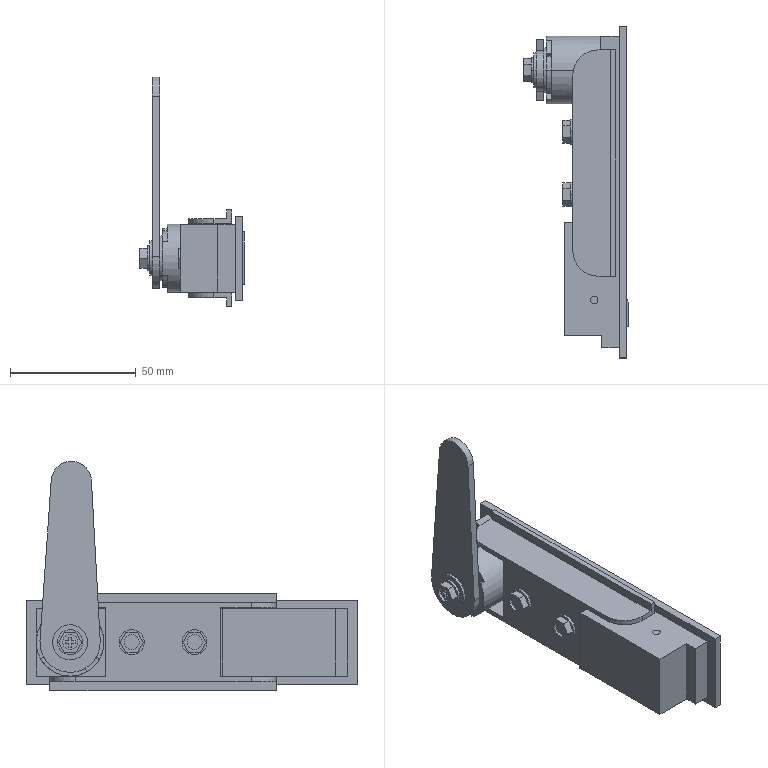Part | SolidWorks | 2 solids | 216 faces | box 41.5 x 132 x 91.25 mm | volume 70272 mm3 | plane 144 | cylinder 62 | cone 8 | torus 2 | commonest cylinder face diameters 3 x8 6 x7 10 x6 22 x5 4.134 x4 5 x4